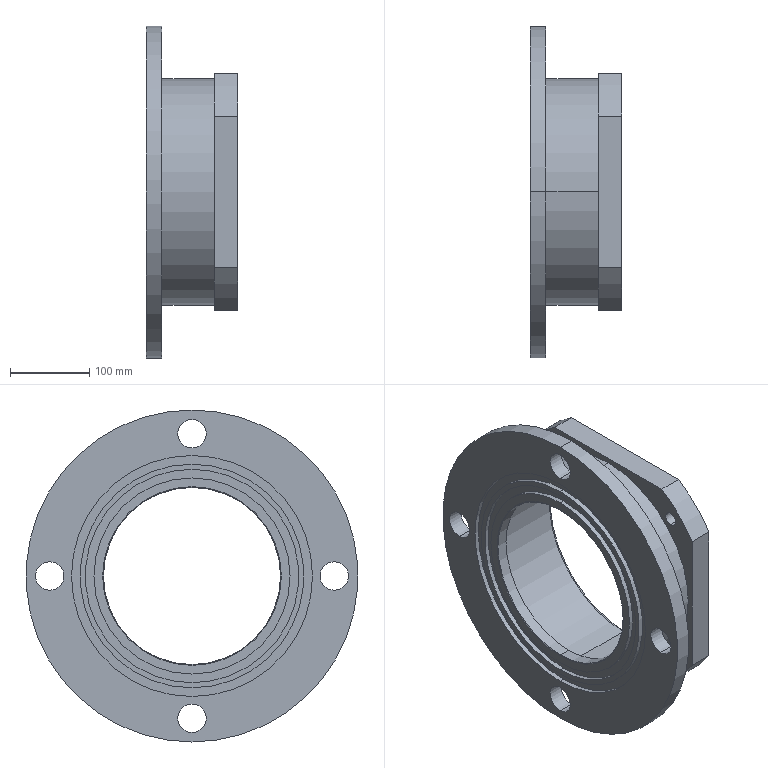Part | SolidWorks | features ICE 4, Chamfer 2, CirPattern 2, HoleWzd 1, RefAxis 1, Revolution 1 | 1 solid | 53 faces | box 116 x 420 x 420 mm | volume 3215271 mm3 | cylinder 36 | plane 13 | cone 4 | commonest cylinder face diameters 17.5 x8 36 x8 356 x4 224 x2 248 x2 264 x2